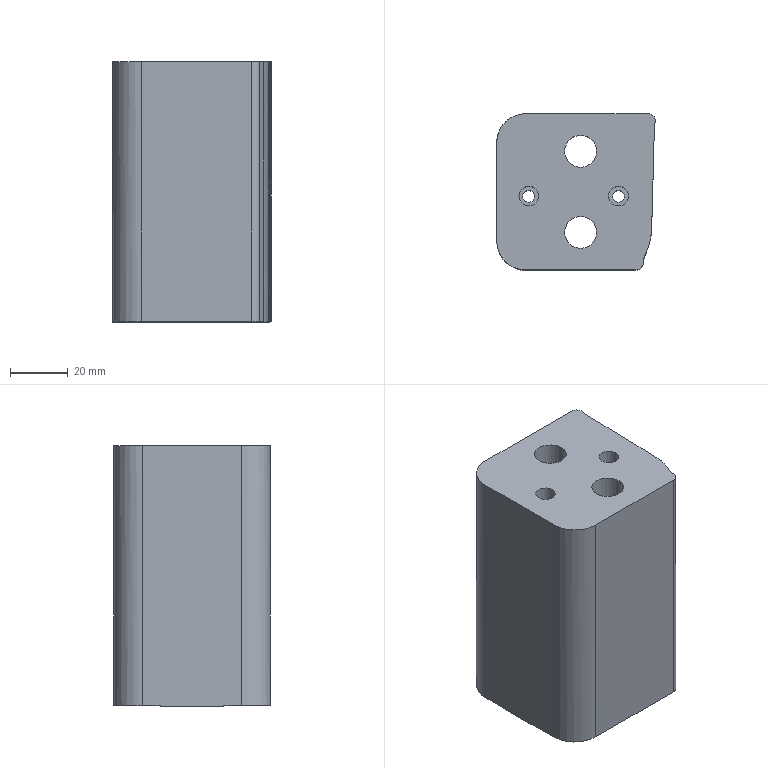Part | STEP file | gslz 2016.10.28-10_id2906_x_t | 1 solid | 30 faces | box 54.788 x 54 x 90 mm | volume 215113 mm3 | cylinder 14 | plane 13 | other 3 | commonest cylinder face diameters 5 x4 4.1 x2 6.8 x2 11 x2 17 x2 20 x2